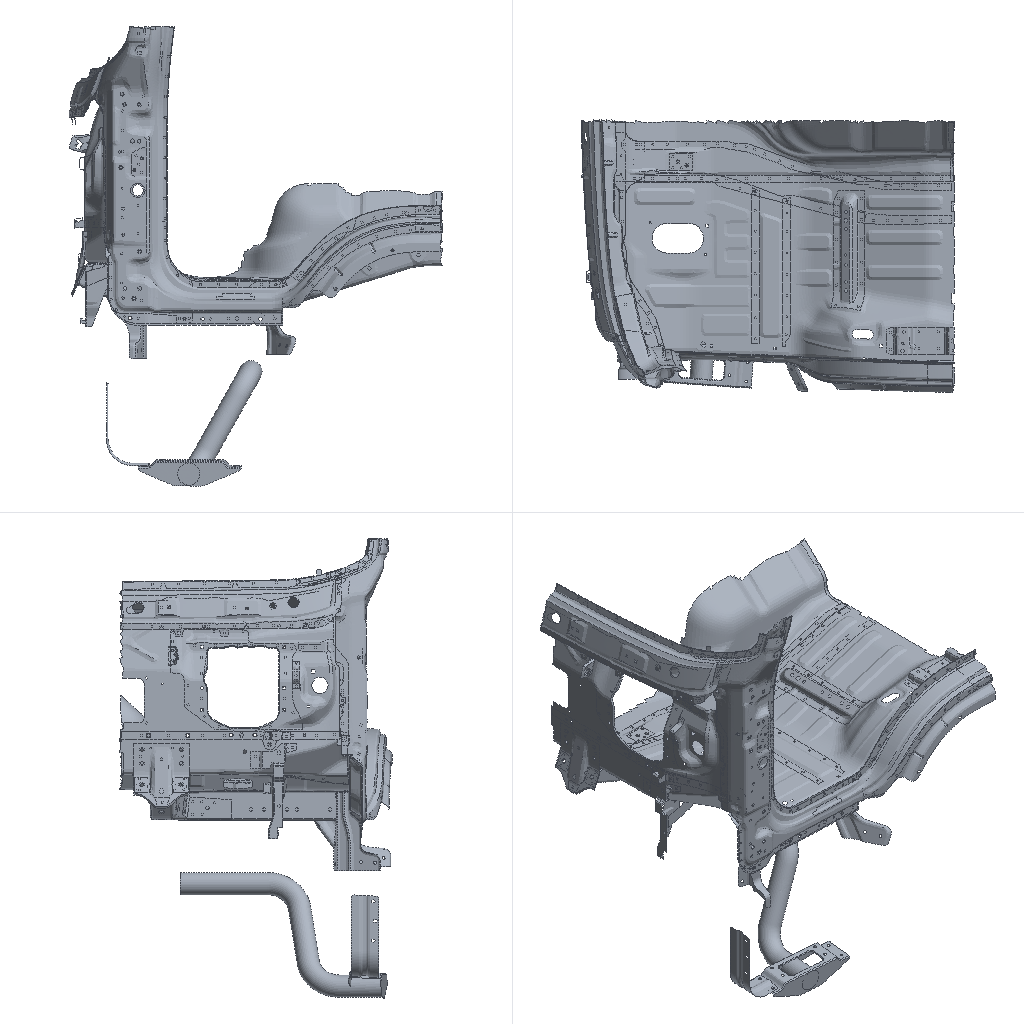Simulation study | nastran
Set-up summary:
category,name,step,type,value,unit,region
solver,nx_nastran
units,not stated in the deck,,not stated
analysis,deck,,static,static
analysis,solution,,SOL,101
load_step,SUBCASE 5,5,SUBCASE,SPC=6 LOAD=7
load_step,requested,,,1
mesh,nodes,,,66623
mesh,elements,,,60711
element_type,CHEXA,,unverified,429
element_type,CQUAD4,,shell,57553
element_type,CTRIA3,,shell,3158
load,nodal force total,,FX,0.0,model units
load,nodal force total,,FY,1470.0,model units
load,nodal force total,,FZ,-2546.12,model units
load,load commands in deck,,count,2
bc,support commands in deck,,count,1155
check,setup vs results,,match,"every grid point's frame and coordinates and every element id; grid points of CHEXA, CQUAD4, CTRIA3 elements"
Nastran input file, long lists of numbers shortened:
$$------------------------------------------------------------------------------$
$$                                                                              $
$$ NASTRAN Input Deck Generated by HyperMesh Version  : 9.0b121                 $
$$ Generated using HyperMesh-Nastran Template Version : 9.0b121
$$                                                                              $
$$   Template:  general                                                         $
$$                                                                              $
$$------------------------------------------------------------------------------$
$$------------------------------------------------------------------------------$
$$                      Executive Control Cards                                 $
$$------------------------------------------------------------------------------$
SOL 101
CEND
$$------------------------------------------------------------------------------$
$$                      Case Control Cards                                      $
$$------------------------------------------------------------------------------$
  DISPLACEMENT(PLOT) = ALL
  STRESS(PLOT) = ALL
$
$HMNAME LOADSTEP               5"step"
SUBCASE       5
  LABEL=    step
  SPC =        6
  LOAD =        7
$$------------------------------------------------------------------------------$
$$                      Bulk Data Cards                                         $
$$------------------------------------------------------------------------------$
BEGIN BULK
PARAM,BAILOUT,-1
PARAM,POST,-1
$$
$$  GRID Data
$$
GRID          27        -966.948-981.428-368.197
GRID          28        -965.765-985.658-368.418
$ (66621 more lines like these left out)
$$
$$  SPOINT Data
$$
$$
$$------------------------------------------------------------------------------$
$$             Group Definitions                                                $
$$------------------------------------------------------------------------------$
$
$ RBE2 Elements - Single dependent node
$
RBE2       14908    8608  123456    2453
RBE2       14909    8607  123456    2452
$ (64 more lines like these left out)
$
$HMMOVE       28
$          14908THRU       14913   14916THRU       14921   14923THRU       14934
$          14936THRU       14943   14945   14947THRU       14949  349213THRU
$         349219  349222THRU      349233
$
$
$HMMOVE 57005014
$         346590  346592THRU      346597  346600THRU      346603
$
$$
$$ RBE2 Elements - Multiple dependent nodes
$$
RBE2       14915    1053  123456    8371    8602
RBE2       14922    1060  123456    8069    8364
$ (146 more lines like these left out)
$
$HMMOVE       28
$          14915   14922   14935   14944  349206THRU      349212  349221  846966
$       THRU      846970
$
$
$HMMOVE 57005014
$         346588THRU      346589  346591  346598THRU      346599  346625THRU
$         346630  346920
$
$
$  RBE3 Elements
$
RBE3      326877         3755976  1234560.226688     123 36403440.012999+
+            123 36403480.041235     123 36403470.719078     123 3640343
RBE3      326878         3755977  1234560.883118     123 36403440.013036+
+            123 36403480.00151      123 36403470.102336     123 3640343
$ (6860 more lines like these left out)
$
$HMMOVE 57005012
$         326877THRU      326880  326882THRU      326889  326891THRU      326898
$         326900THRU      326907  326909THRU      326916  326918THRU      326925
$ (169 more lines like these left out)
CTRIA3     16839      16   16998   16997   17043
CTRIA3     17868      16   17974   17986   17973
$ (3156 more lines like these left out)
$
$HMMOVE        2
$          16839   17868   17934   17953   17973
$
$ (375 more lines like these left out)
CQUAD4     16155      16   16324   16261   16262   16323
CQUAD4     16156      16   16323   16262   16263   16322
$ (57551 more lines like these left out)
$
$HMMOVE        2
$          16155THRU       16390   16561THRU       16838   16840THRU       16848
$          16851THRU       16852   16855THRU       16856   16860THRU       16861
$ (1121 more lines like these left out)
CHEXA     326881      10 3755976 3755979 3755978 3755977 3755980 3755983+
+        3755982 3755981
CHEXA     326890      10 3755985 3755988 3755987 3755986 3755989 3755992+
+        3755991 3755990
$ (854 more lines like these left out)
$
$HMMOVE 57005011
$         326881  326890  326899  326908  326917  326926  326935  326944  326953
$         326962  326971  326980  326989  326998  327007  327016  327025  327034
$ (204 more lines like these left out)
PSHELL         4       11.0            1               1
$
$HMNAME PROP                   5"150" 4
$HWCOLOR PROP                  5       3
PSHELL         5       11.5            1               1
$
$HMNAME PROP                   6"250" 4
$HWCOLOR PROP                  6       3
PSHELL         6       12.5            1               1
$
$HMNAME PROP                   7"200" 4
$HWCOLOR PROP                  7       3
PSHELL         7       12.0            1               1
$
$HMNAME PROP                  16"Sheel_300T" 4
$HWCOLOR PROP                 16       3
PSHELL        16      353.0           35              35
$
$HMNAME PROP                   8"160" 4
$HWCOLOR PROP                  8       3
PSHELL         8       11.6            1               1
$
$HMNAME PROP                   3"180" 4
$HWCOLOR PROP                  3       3
PSHELL         3       11.8            1               1
$
$HMNAME PROP                   2"120" 4
$HWCOLOR PROP                  2       3
PSHELL         2       11.2            1               1
$
$
$
$HMNAME PROP                   1"80" 4
$HWCOLOR PROP                  1       3
PSHELL         1       10.8            1               1
$
$HMNAME PROP                  11"Sheel_300T.1" 4
$HWCOLOR PROP                 11       3
PSHELL        11       13.0            1               1
$
$HMNAME PROP                  12"Sheel_350T" 4
$HWCOLOR PROP                 12       4
PSHELL        12       13.5            1               1
$
$HMNAME PROP                  13"Sheel_500T" 4
$HWCOLOR PROP                 13       5
PSHELL        13       15.0            1               1
$$
$$  PSOLID Data
$
$HMNAME PROP                  10"spot" 5
$HWCOLOR PROP                 10       3
PSOLID        10       1
$$
$$------------------------------------------------------------------------------$
$$                      Material Definition Cards                               $
$$------------------------------------------------------------------------------$
$$--------------------------------------------------------------
$$ HYPERMESH TAGS
$$--------------------------------------------------------------
$$BEGIN TAGS
$$END TAGS
$$
$$  MAT1 Data
$
$HMNAME MAT                   35"Steel" "MAT1"
$HWCOLOR MAT                  35       6
MAT1          35210000.0        0.3     7.80E-09
$
$HMNAME MAT                    1"steel" "MAT1"
$HWCOLOR MAT                   1       3
MAT1           1210000.0        0.3     7.90E-09
$$
$$
$$
$$------------------------------------------------------------------------------$
$ (37 more lines like these left out)
SPC            6  103169  1234560.0
SPC            6  103168  1234560.0
SPC            6  103166  1234560.0
SPC            6  103161  1234560.0
$ (1151 more lines like these left out)
$$
$$  FORCE Data
$$
FORCE          784121622       01.0     0.0     735.0   -1273.06
FORCE          784121623       01.0     0.0     735.0   -1273.06
$HMASSEM   28010       3 2801
$HMASSEM   28011       3 tabu
$HMASSEM_IDS           2
$HMASSEM 5400100       7 sidebody_L
$HMASSEM_IDS    5400101054003020540011105400112054003010
$HMASSEM      28       4 5300010
$HMASSEM_IDS          16      18      20      21      22      24      25      26
$HMASSEM 5700101       3 tabu.1
$HMASSEM_IDS          238402269384022695      27
$HMASSEM       1       3 REAR_FLOOR
$HMASSEM_IDS    5100990051003010510033105100111051005210510012105100521151005510
$HMASSEM_IDS    5100141051009310510045105100421051004811510043115100541051007010
$HMASSEM_IDS    51007210510056105100561151004310510050105100341051009711
$
ENDDATA
Results summary:
result,analysis,,,static
result,last_loadstep,,,1
result,primary field,,,displacements
result,max displacement,,,2.026,model units